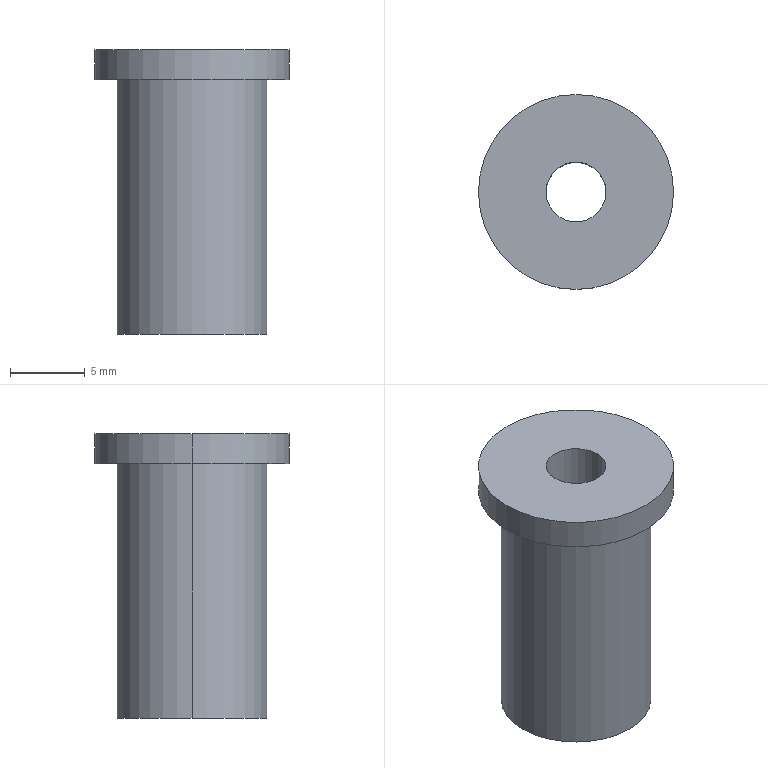Part | STEP file | 11-FG-B04211 | 1 solid | 9 faces | box 13 x 13 x 19 mm | volume 1362 mm3 | cylinder 6 | plane 3 | commonest cylinder face diameters 4 x2 10 x2 13 x2
STEP:
#1=CARTESIAN_POINT('',(6.5,0.,19.));
#2=VERTEX_POINT('',#1);
#3=CARTESIAN_POINT('',(-6.5,0.,19.));
#4=VERTEX_POINT('',#3);
#5=CARTESIAN_POINT('',(0.,0.,19.));
#6=DIRECTION('',(0.,0.,1.));
#7=DIRECTION('',(1.,0.,0.));
#8=AXIS2_PLACEMENT_3D('',#5,#6,#7);
#9=CIRCLE('',#8,6.5);
#10=EDGE_CURVE('',#2,#4,#9,.T.);
#11=ORIENTED_EDGE('',*,*,#10,.F.);
#12=CARTESIAN_POINT('',(6.5,0.,17.));
#13=VERTEX_POINT('',#12);
#14=CARTESIAN_POINT('',(6.5,0.,19.));
#15=DIRECTION('',(0.,0.,-1.));
#16=VECTOR('',#15,1000.);
#17=LINE('',#14,#16);
#18=EDGE_CURVE('',#2,#13,#17,.T.);
#19=ORIENTED_EDGE('',*,*,#18,.T.);
#20=CARTESIAN_POINT('',(-6.5,0.,17.));
#21=VERTEX_POINT('',#20);
#22=CARTESIAN_POINT('',(0.,0.,17.));
#23=DIRECTION('',(0.,0.,1.));
#24=DIRECTION('',(1.,0.,0.));
#25=AXIS2_PLACEMENT_3D('',#22,#23,#24);
#26=CIRCLE('',#25,6.5);
#27=EDGE_CURVE('',#13,#21,#26,.T.);
#28=ORIENTED_EDGE('',*,*,#27,.T.);
#29=CARTESIAN_POINT('',(-6.5,0.,19.));
#30=DIRECTION('',(0.,0.,-1.));
#31=VECTOR('',#30,1000.);
#32=LINE('',#29,#31);
#33=EDGE_CURVE('',#4,#21,#32,.T.);
#34=ORIENTED_EDGE('',*,*,#33,.F.);
#35=EDGE_LOOP('',(#11,#19,#28,#34));
#36=FACE_OUTER_BOUND('',#35,.T.);
#37=CARTESIAN_POINT('',(0.,0.,19.));
#38=DIRECTION('',(0.,0.,-1.));
#39=DIRECTION('',(-1.,0.,0.));
#40=AXIS2_PLACEMENT_3D('',#37,#38,#39);
#41=CYLINDRICAL_SURFACE('',#40,6.5);
#42=ADVANCED_FACE('',(#36),#41,.T.);
#43=CARTESIAN_POINT('',(-2.,0.,19.));
#44=VERTEX_POINT('',#43);
#45=CARTESIAN_POINT('',(2.,0.,19.));
#46=VERTEX_POINT('',#45);
#47=CARTESIAN_POINT('',(0.,0.,19.));
#48=DIRECTION('',(0.,0.,1.));
#49=DIRECTION('',(1.,0.,0.));
#50=AXIS2_PLACEMENT_3D('',#47,#48,#49);
#51=CIRCLE('',#50,2.);
#52=EDGE_CURVE('',#44,#46,#51,.T.);
#53=ORIENTED_EDGE('',*,*,#52,.T.);
#54=CARTESIAN_POINT('',(2.,0.,0.));
#55=VERTEX_POINT('',#54);
#56=CARTESIAN_POINT('',(2.,0.,17.));
#57=DIRECTION('',(0.,0.,-1.));
#58=VECTOR('',#57,1000.);
#59=LINE('',#56,#58);
#60=EDGE_CURVE('',#46,#55,#59,.T.);
#61=ORIENTED_EDGE('',*,*,#60,.T.);
#62=CARTESIAN_POINT('',(-2.,0.,0.));
#63=VERTEX_POINT('',#62);
#64=CARTESIAN_POINT('',(0.,0.,0.));
#65=DIRECTION('',(0.,0.,1.));
#66=DIRECTION('',(1.,0.,0.));
#67=AXIS2_PLACEMENT_3D('',#64,#65,#66);
#68=CIRCLE('',#67,2.);
#69=EDGE_CURVE('',#63,#55,#68,.T.);
#70=ORIENTED_EDGE('',*,*,#69,.F.);
#71=CARTESIAN_POINT('',(-2.,0.,17.));
#72=DIRECTION('',(0.,0.,-1.));
#73=VECTOR('',#72,1000.);
#74=LINE('',#71,#73);
#75=EDGE_CURVE('',#44,#63,#74,.T.);
#76=ORIENTED_EDGE('',*,*,#75,.F.);
#77=EDGE_LOOP('',(#53,#61,#70,#76));
#78=FACE_OUTER_BOUND('',#77,.T.);
#79=CARTESIAN_POINT('',(0.,0.,17.));
#80=DIRECTION('',(0.,0.,-1.));
#81=DIRECTION('',(-1.,0.,0.));
#82=AXIS2_PLACEMENT_3D('',#79,#80,#81);
#83=CYLINDRICAL_SURFACE('',#82,2.);
#84=ADVANCED_FACE('',(#78),#83,.F.);
#85=CARTESIAN_POINT('',(5.,0.,17.));
#86=VERTEX_POINT('',#85);
#87=CARTESIAN_POINT('',(-5.,0.,17.));
#88=VERTEX_POINT('',#87);
#89=CARTESIAN_POINT('',(0.,0.,17.));
#90=DIRECTION('',(0.,0.,1.));
#91=DIRECTION('',(1.,0.,0.));
#92=AXIS2_PLACEMENT_3D('',#89,#90,#91);
#93=CIRCLE('',#92,5.);
#94=EDGE_CURVE('',#86,#88,#93,.T.);
#95=ORIENTED_EDGE('',*,*,#94,.F.);
#96=CARTESIAN_POINT('',(5.,0.,0.));
#97=VERTEX_POINT('',#96);
#98=CARTESIAN_POINT('',(5.,0.,17.));
#99=DIRECTION('',(0.,0.,-1.));
#100=VECTOR('',#99,1000.);
#101=LINE('',#98,#100);
#102=EDGE_CURVE('',#86,#97,#101,.T.);
#103=ORIENTED_EDGE('',*,*,#102,.T.);
#104=CARTESIAN_POINT('',(-5.,0.,0.));
#105=VERTEX_POINT('',#104);
#106=CARTESIAN_POINT('',(0.,0.,0.));
#107=DIRECTION('',(0.,0.,1.));
#108=DIRECTION('',(1.,0.,0.));
#109=AXIS2_PLACEMENT_3D('',#106,#107,#108);
#110=CIRCLE('',#109,5.);
#111=EDGE_CURVE('',#97,#105,#110,.T.);
#112=ORIENTED_EDGE('',*,*,#111,.T.);
#113=CARTESIAN_POINT('',(-5.,0.,17.));
#114=DIRECTION('',(0.,0.,-1.));
#115=VECTOR('',#114,1000.);
#116=LINE('',#113,#115);
#117=EDGE_CURVE('',#88,#105,#116,.T.);
#118=ORIENTED_EDGE('',*,*,#117,.F.);
#119=EDGE_LOOP('',(#95,#103,#112,#118));
#120=FACE_OUTER_BOUND('',#119,.T.);
#121=CARTESIAN_POINT('',(0.,0.,17.));
#122=DIRECTION('',(0.,0.,-1.));
#123=DIRECTION('',(-1.,0.,0.));
#124=AXIS2_PLACEMENT_3D('',#121,#122,#123);
#125=CYLINDRICAL_SURFACE('',#124,5.);
#126=ADVANCED_FACE('',(#120),#125,.T.);
#127=CARTESIAN_POINT('',(0.,0.,0.));
#128=DIRECTION('',(0.,0.,1.));
#129=DIRECTION('',(1.,0.,0.));
#130=AXIS2_PLACEMENT_3D('',#127,#128,#129);
#131=CIRCLE('',#130,5.);
#132=EDGE_CURVE('',#105,#97,#131,.T.);
#133=ORIENTED_EDGE('',*,*,#132,.F.);
#134=ORIENTED_EDGE('',*,*,#111,.F.);
#135=EDGE_LOOP('',(#133,#134));
#136=FACE_OUTER_BOUND('',#135,.T.);
#137=ORIENTED_EDGE('',*,*,#69,.T.);
#138=CARTESIAN_POINT('',(0.,0.,0.));
#139=DIRECTION('',(0.,0.,1.));
#140=DIRECTION('',(1.,0.,0.));
#141=AXIS2_PLACEMENT_3D('',#138,#139,#140);
#142=CIRCLE('',#141,2.);
#143=EDGE_CURVE('',#55,#63,#142,.T.);
#144=ORIENTED_EDGE('',*,*,#143,.T.);
#145=EDGE_LOOP('',(#137,#144));
#146=FACE_BOUND('',#145,.T.);
#147=CARTESIAN_POINT('',(0.,0.,0.));
#148=DIRECTION('',(0.,0.,1.));
#149=DIRECTION('',(1.,0.,0.));
#150=AXIS2_PLACEMENT_3D('',#147,#148,#149);
#151=PLANE('',#150);
#152=ADVANCED_FACE('',(#136,#146),#151,.F.);
#153=ORIENTED_EDGE('',*,*,#102,.F.);
#154=CARTESIAN_POINT('',(0.,0.,17.));
#155=DIRECTION('',(0.,0.,1.));
#156=DIRECTION('',(1.,0.,0.));
#157=AXIS2_PLACEMENT_3D('',#154,#155,#156);
#158=CIRCLE('',#157,5.);
#159=EDGE_CURVE('',#88,#86,#158,.T.);
#160=ORIENTED_EDGE('',*,*,#159,.F.);
#161=ORIENTED_EDGE('',*,*,#117,.T.);
#162=ORIENTED_EDGE('',*,*,#132,.T.);
#163=EDGE_LOOP('',(#153,#160,#161,#162));
#164=FACE_OUTER_BOUND('',#163,.T.);
#165=CARTESIAN_POINT('',(0.,0.,17.));
#166=DIRECTION('',(0.,0.,-1.));
#167=DIRECTION('',(-1.,0.,0.));
#168=AXIS2_PLACEMENT_3D('',#165,#166,#167);
#169=CYLINDRICAL_SURFACE('',#168,5.);
#170=ADVANCED_FACE('',(#164),#169,.T.);
#171=ORIENTED_EDGE('',*,*,#60,.F.);
#172=CARTESIAN_POINT('',(0.,0.,19.));
#173=DIRECTION('',(0.,0.,1.));
#174=DIRECTION('',(1.,0.,0.));
#175=AXIS2_PLACEMENT_3D('',#172,#173,#174);
#176=CIRCLE('',#175,2.);
#177=EDGE_CURVE('',#46,#44,#176,.T.);
#178=ORIENTED_EDGE('',*,*,#177,.T.);
#179=ORIENTED_EDGE('',*,*,#75,.T.);
#180=ORIENTED_EDGE('',*,*,#143,.F.);
#181=EDGE_LOOP('',(#171,#178,#179,#180));
#182=FACE_OUTER_BOUND('',#181,.T.);
#183=CARTESIAN_POINT('',(0.,0.,17.));
#184=DIRECTION('',(0.,0.,-1.));
#185=DIRECTION('',(-1.,0.,0.));
#186=AXIS2_PLACEMENT_3D('',#183,#184,#185);
#187=CYLINDRICAL_SURFACE('',#186,2.);
#188=ADVANCED_FACE('',(#182),#187,.F.);
#189=CARTESIAN_POINT('',(0.,0.,17.));
#190=DIRECTION('',(0.,0.,1.));
#191=DIRECTION('',(1.,0.,0.));
#192=AXIS2_PLACEMENT_3D('',#189,#190,#191);
#193=CIRCLE('',#192,6.5);
#194=EDGE_CURVE('',#21,#13,#193,.T.);
#195=ORIENTED_EDGE('',*,*,#194,.F.);
#196=ORIENTED_EDGE('',*,*,#27,.F.);
#197=EDGE_LOOP('',(#195,#196));
#198=FACE_OUTER_BOUND('',#197,.T.);
#199=ORIENTED_EDGE('',*,*,#159,.T.);
#200=ORIENTED_EDGE('',*,*,#94,.T.);
#201=EDGE_LOOP('',(#199,#200));
#202=FACE_BOUND('',#201,.T.);
#203=CARTESIAN_POINT('',(0.,0.,17.));
#204=DIRECTION('',(0.,0.,1.));
#205=DIRECTION('',(1.,0.,0.));
#206=AXIS2_PLACEMENT_3D('',#203,#204,#205);
#207=PLANE('',#206);
#208=ADVANCED_FACE('',(#198,#202),#207,.F.);
#209=CARTESIAN_POINT('',(0.,0.,19.));
#210=DIRECTION('',(0.,0.,1.));
#211=DIRECTION('',(1.,0.,0.));
#212=AXIS2_PLACEMENT_3D('',#209,#210,#211);
#213=CIRCLE('',#212,6.5);
#214=EDGE_CURVE('',#4,#2,#213,.T.);
#215=ORIENTED_EDGE('',*,*,#214,.T.);
#216=ORIENTED_EDGE('',*,*,#10,.T.);
#217=EDGE_LOOP('',(#215,#216));
#218=FACE_OUTER_BOUND('',#217,.T.);
#219=ORIENTED_EDGE('',*,*,#52,.F.);
#220=ORIENTED_EDGE('',*,*,#177,.F.);
#221=EDGE_LOOP('',(#219,#220));
#222=FACE_BOUND('',#221,.T.);
#223=CARTESIAN_POINT('',(0.,0.,19.));
#224=DIRECTION('',(0.,0.,1.));
#225=DIRECTION('',(1.,0.,0.));
#226=AXIS2_PLACEMENT_3D('',#223,#224,#225);
#227=PLANE('',#226);
#228=ADVANCED_FACE('',(#218,#222),#227,.T.);
#229=ORIENTED_EDGE('',*,*,#18,.F.);
#230=ORIENTED_EDGE('',*,*,#214,.F.);
#231=ORIENTED_EDGE('',*,*,#33,.T.);
#232=ORIENTED_EDGE('',*,*,#194,.T.);
#233=EDGE_LOOP('',(#229,#230,#231,#232));
#234=FACE_OUTER_BOUND('',#233,.T.);
#235=CARTESIAN_POINT('',(0.,0.,19.));
#236=DIRECTION('',(0.,0.,-1.));
#237=DIRECTION('',(-1.,0.,0.));
#238=AXIS2_PLACEMENT_3D('',#235,#236,#237);
#239=CYLINDRICAL_SURFACE('',#238,6.5);
#240=ADVANCED_FACE('',(#234),#239,.T.);
#241=CLOSED_SHELL('',(#42,#84,#126,#152,#170,#188,#208,#228,#240));
#242=MANIFOLD_SOLID_BREP('',#241);
#243=CARTESIAN_POINT('',(0.,0.,0.));
#244=DIRECTION('',(0.,0.,1.));
#245=DIRECTION('',(1.,0.,0.));
#246=AXIS2_PLACEMENT_3D('',#243,#244,#245);
#247=(LENGTH_UNIT()NAMED_UNIT(*)SI_UNIT(.MILLI.,.METRE.));
#248=UNCERTAINTY_MEASURE_WITH_UNIT(LENGTH_MEASURE(0.00001),#247,'','');
#249=(NAMED_UNIT(*)PLANE_ANGLE_UNIT()SI_UNIT($,.RADIAN.));
#250=(NAMED_UNIT(*)SI_UNIT($,.STERADIAN.)SOLID_ANGLE_UNIT());
#251=(GEOMETRIC_REPRESENTATION_CONTEXT(3)GLOBAL_UNCERTAINTY_ASSIGNED_CONTEXT((#248))GLOBAL_UNIT_ASSIGNED_CONTEXT((#247,#249,#250))REPRESENTATION_CONTEXT('',''));
#252=ADVANCED_BREP_SHAPE_REPRESENTATION('',(#242,#246),#251);